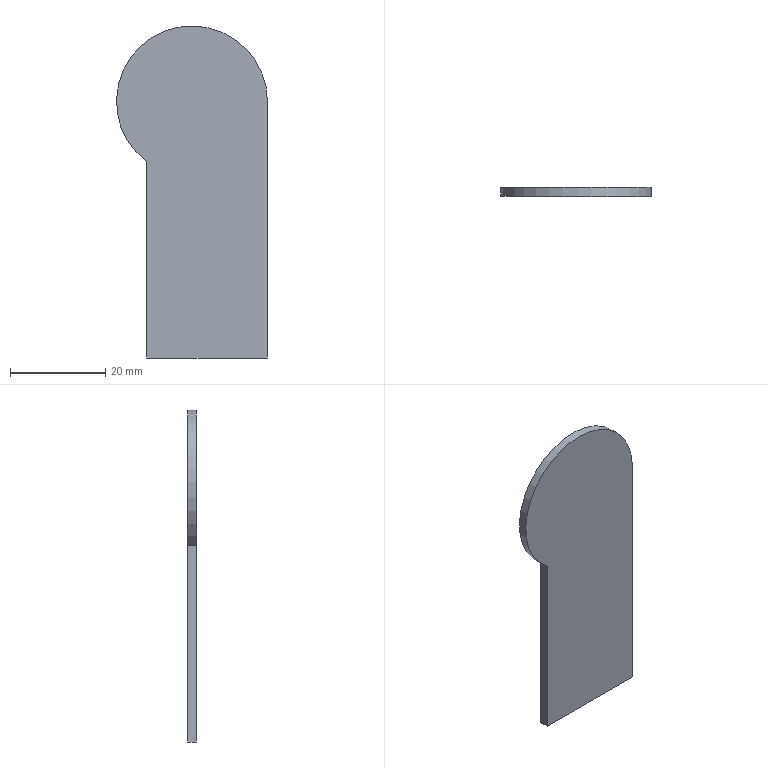Part | NX | features BREP 1 | 1 solid | 6 faces | box 31.75 x 1.88 x 69.85 mm | volume 3427 mm3 | plane 5 | cylinder 1 | commonest cylinder face diameters 31.75 x1
STEP:
#1=CARTESIAN_POINT('',(-12.7,0.,-12.7));
#2=VERTEX_POINT('',#1);
#3=CARTESIAN_POINT('',(12.7,0.,0.));
#4=VERTEX_POINT('',#3);
#5=CARTESIAN_POINT('',(-3.175,0.,0.));
#6=DIRECTION('',(0.,1.,0.));
#7=DIRECTION('',(-0.6,0.,-0.8));
#8=AXIS2_PLACEMENT_3D('',#5,#6,#7);
#9=CIRCLE('',#8,15.875);
#10=EDGE_CURVE('',#2,#4,#9,.T.);
#11=ORIENTED_EDGE('',*,*,#10,.T.);
#12=CARTESIAN_POINT('',(12.7,0.,-53.975));
#13=VERTEX_POINT('',#12);
#14=CARTESIAN_POINT('',(12.7,0.,0.));
#15=DIRECTION('',(0.,0.,-1.));
#16=VECTOR('',#15,1000.);
#17=LINE('',#14,#16);
#18=EDGE_CURVE('',#4,#13,#17,.T.);
#19=ORIENTED_EDGE('',*,*,#18,.T.);
#20=CARTESIAN_POINT('',(-12.7,0.,-53.975));
#21=VERTEX_POINT('',#20);
#22=CARTESIAN_POINT('',(12.7,0.,-53.975));
#23=DIRECTION('',(-1.,0.,0.));
#24=VECTOR('',#23,1000.);
#25=LINE('',#22,#24);
#26=EDGE_CURVE('',#13,#21,#25,.T.);
#27=ORIENTED_EDGE('',*,*,#26,.T.);
#28=CARTESIAN_POINT('',(-12.7,0.,-53.975));
#29=DIRECTION('',(0.,0.,1.));
#30=VECTOR('',#29,1000.);
#31=LINE('',#28,#30);
#32=EDGE_CURVE('',#21,#2,#31,.T.);
#33=ORIENTED_EDGE('',*,*,#32,.T.);
#34=EDGE_LOOP('',(#11,#19,#27,#33));
#35=FACE_BOUND('',#34,.T.);
#36=CARTESIAN_POINT('',(0.,0.,0.));
#37=DIRECTION('',(0.,1.,0.));
#38=DIRECTION('',(1.,0.,0.));
#39=AXIS2_PLACEMENT_3D('',#36,#37,#38);
#40=PLANE('',#39);
#41=ADVANCED_FACE('',(#35),#40,.T.);
#42=CARTESIAN_POINT('',(-12.7,-1.88,-53.975));
#43=VERTEX_POINT('',#42);
#44=CARTESIAN_POINT('',(-12.7,0.,-53.975));
#45=DIRECTION('',(0.,-1.,0.));
#46=VECTOR('',#45,1000.);
#47=LINE('',#44,#46);
#48=EDGE_CURVE('',#21,#43,#47,.T.);
#49=ORIENTED_EDGE('',*,*,#48,.T.);
#50=CARTESIAN_POINT('',(-12.7,-1.88,-12.7));
#51=VERTEX_POINT('',#50);
#52=CARTESIAN_POINT('',(-12.7,-1.88,-53.975));
#53=DIRECTION('',(0.,0.,1.));
#54=VECTOR('',#53,1000.);
#55=LINE('',#52,#54);
#56=EDGE_CURVE('',#43,#51,#55,.T.);
#57=ORIENTED_EDGE('',*,*,#56,.T.);
#58=CARTESIAN_POINT('',(-12.7,0.,-12.7));
#59=DIRECTION('',(0.,-1.,0.));
#60=VECTOR('',#59,1000.);
#61=LINE('',#58,#60);
#62=EDGE_CURVE('',#2,#51,#61,.T.);
#63=ORIENTED_EDGE('',*,*,#62,.F.);
#64=ORIENTED_EDGE('',*,*,#32,.F.);
#65=EDGE_LOOP('',(#49,#57,#63,#64));
#66=FACE_BOUND('',#65,.T.);
#67=CARTESIAN_POINT('',(-12.7,-0.9398,-33.337));
#68=DIRECTION('',(-1.,0.,0.));
#69=DIRECTION('',(0.,0.,1.));
#70=AXIS2_PLACEMENT_3D('',#67,#68,#69);
#71=PLANE('',#70);
#72=ADVANCED_FACE('',(#66),#71,.T.);
#73=ORIENTED_EDGE('',*,*,#62,.T.);
#74=CARTESIAN_POINT('',(12.7,-1.88,0.));
#75=VERTEX_POINT('',#74);
#76=CARTESIAN_POINT('',(-3.175,-1.88,0.));
#77=DIRECTION('',(0.,1.,0.));
#78=DIRECTION('',(-0.6,0.,-0.8));
#79=AXIS2_PLACEMENT_3D('',#76,#77,#78);
#80=CIRCLE('',#79,15.875);
#81=EDGE_CURVE('',#51,#75,#80,.T.);
#82=ORIENTED_EDGE('',*,*,#81,.T.);
#83=CARTESIAN_POINT('',(12.7,0.,0.));
#84=DIRECTION('',(0.,-1.,0.));
#85=VECTOR('',#84,1000.);
#86=LINE('',#83,#85);
#87=EDGE_CURVE('',#4,#75,#86,.T.);
#88=ORIENTED_EDGE('',*,*,#87,.F.);
#89=ORIENTED_EDGE('',*,*,#10,.F.);
#90=EDGE_LOOP('',(#73,#82,#88,#89));
#91=FACE_BOUND('',#90,.T.);
#92=CARTESIAN_POINT('',(-3.175,-0.9398,0.));
#93=DIRECTION('',(0.,1.,0.));
#94=DIRECTION('',(-0.6,0.,-0.8));
#95=AXIS2_PLACEMENT_3D('',#92,#93,#94);
#96=CYLINDRICAL_SURFACE('',#95,15.875);
#97=ADVANCED_FACE('',(#91),#96,.T.);
#98=ORIENTED_EDGE('',*,*,#87,.T.);
#99=CARTESIAN_POINT('',(12.7,-1.88,-53.975));
#100=VERTEX_POINT('',#99);
#101=CARTESIAN_POINT('',(12.7,-1.88,0.));
#102=DIRECTION('',(0.,0.,-1.));
#103=VECTOR('',#102,1000.);
#104=LINE('',#101,#103);
#105=EDGE_CURVE('',#75,#100,#104,.T.);
#106=ORIENTED_EDGE('',*,*,#105,.T.);
#107=CARTESIAN_POINT('',(12.7,0.,-53.975));
#108=DIRECTION('',(0.,-1.,0.));
#109=VECTOR('',#108,1000.);
#110=LINE('',#107,#109);
#111=EDGE_CURVE('',#13,#100,#110,.T.);
#112=ORIENTED_EDGE('',*,*,#111,.F.);
#113=ORIENTED_EDGE('',*,*,#18,.F.);
#114=EDGE_LOOP('',(#98,#106,#112,#113));
#115=FACE_BOUND('',#114,.T.);
#116=CARTESIAN_POINT('',(12.7,-0.9398,-26.988));
#117=DIRECTION('',(1.,0.,0.));
#118=DIRECTION('',(0.,1.,0.));
#119=AXIS2_PLACEMENT_3D('',#116,#117,#118);
#120=PLANE('',#119);
#121=ADVANCED_FACE('',(#115),#120,.T.);
#122=ORIENTED_EDGE('',*,*,#111,.T.);
#123=CARTESIAN_POINT('',(12.7,-1.88,-53.975));
#124=DIRECTION('',(-1.,0.,0.));
#125=VECTOR('',#124,1000.);
#126=LINE('',#123,#125);
#127=EDGE_CURVE('',#100,#43,#126,.T.);
#128=ORIENTED_EDGE('',*,*,#127,.T.);
#129=ORIENTED_EDGE('',*,*,#48,.F.);
#130=ORIENTED_EDGE('',*,*,#26,.F.);
#131=EDGE_LOOP('',(#122,#128,#129,#130));
#132=FACE_BOUND('',#131,.T.);
#133=CARTESIAN_POINT('',(0.,-0.9398,-53.975));
#134=DIRECTION('',(0.,0.,-1.));
#135=DIRECTION('',(0.,-1.,0.));
#136=AXIS2_PLACEMENT_3D('',#133,#134,#135);
#137=PLANE('',#136);
#138=ADVANCED_FACE('',(#132),#137,.T.);
#139=ORIENTED_EDGE('',*,*,#127,.F.);
#140=ORIENTED_EDGE('',*,*,#105,.F.);
#141=ORIENTED_EDGE('',*,*,#81,.F.);
#142=ORIENTED_EDGE('',*,*,#56,.F.);
#143=EDGE_LOOP('',(#139,#140,#141,#142));
#144=FACE_BOUND('',#143,.T.);
#145=CARTESIAN_POINT('',(0.,-1.88,0.));
#146=DIRECTION('',(0.,1.,0.));
#147=DIRECTION('',(1.,0.,0.));
#148=AXIS2_PLACEMENT_3D('',#145,#146,#147);
#149=PLANE('',#148);
#150=ADVANCED_FACE('',(#144),#149,.F.);
#151=CLOSED_SHELL('',(#41,#72,#97,#121,#138,#150));
#152=MANIFOLD_SOLID_BREP('',#151);
#153=(LENGTH_UNIT()NAMED_UNIT(*)SI_UNIT(.MILLI.,.METRE.));
#154=UNCERTAINTY_MEASURE_WITH_UNIT(LENGTH_MEASURE(0.00001),#153,'','');
#155=(NAMED_UNIT(*)PLANE_ANGLE_UNIT()SI_UNIT($,.RADIAN.));
#156=(NAMED_UNIT(*)SI_UNIT($,.STERADIAN.)SOLID_ANGLE_UNIT());
#157=(GEOMETRIC_REPRESENTATION_CONTEXT(3)GLOBAL_UNCERTAINTY_ASSIGNED_CONTEXT((#154))GLOBAL_UNIT_ASSIGNED_CONTEXT((#153,#155,#156))REPRESENTATION_CONTEXT('',''));
#158=ADVANCED_BREP_SHAPE_REPRESENTATION('',(#152),#157);